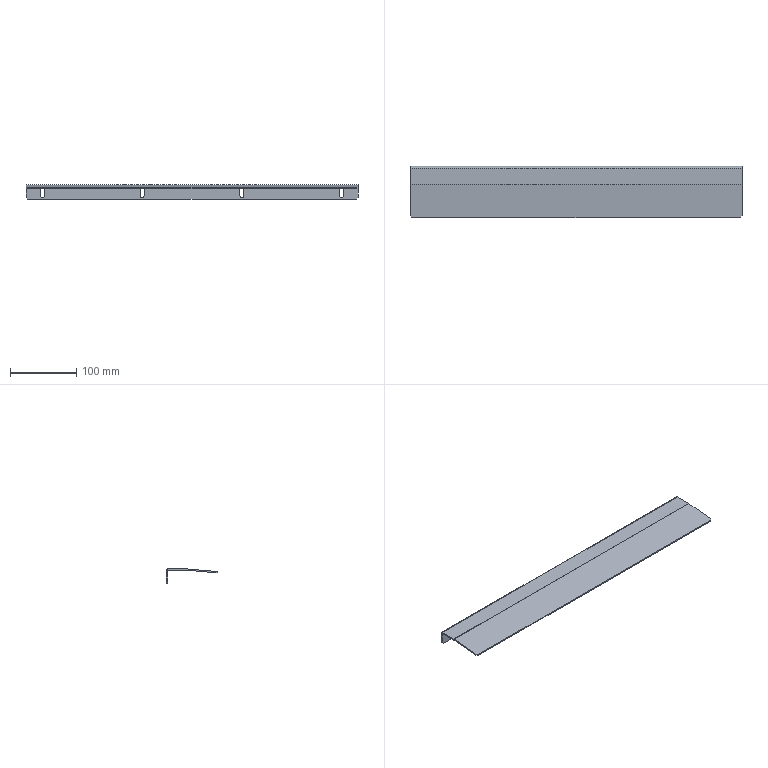Part | NX | 1 solid | 42 faces | box 500 x 76.984 x 22 mm | volume 95676 mm3 | plane 30 | cylinder 12 | commonest cylinder face diameters 5.5 x8 1.473 x2 5.473 x2
STEP:
#1=CARTESIAN_POINT('',(250.,-12.468,-2.));
#2=VERTEX_POINT('',#1);
#3=CARTESIAN_POINT('',(250.,11.763,-2.));
#4=VERTEX_POINT('',#3);
#5=CARTESIAN_POINT('',(250.,-12.5,-2.));
#6=DIRECTION('',(0.,1.,0.));
#7=VECTOR('',#6,1000.);
#8=LINE('',#5,#7);
#9=EDGE_CURVE('',#2,#4,#8,.T.);
#10=ORIENTED_EDGE('',*,*,#9,.F.);
#11=CARTESIAN_POINT('',(-250.,-12.468,-2.));
#12=VERTEX_POINT('',#11);
#13=CARTESIAN_POINT('',(-250.,-12.468,-2.));
#14=DIRECTION('',(-1.,0.,0.));
#15=VECTOR('',#14,1000.);
#16=LINE('',#13,#15);
#17=EDGE_CURVE('',#12,#2,#16,.F.);
#18=ORIENTED_EDGE('',*,*,#17,.F.);
#19=CARTESIAN_POINT('',(-250.,11.763,-2.));
#20=VERTEX_POINT('',#19);
#21=CARTESIAN_POINT('',(-250.,-12.5,-2.));
#22=DIRECTION('',(0.,-1.,0.));
#23=VECTOR('',#22,1000.);
#24=LINE('',#21,#23);
#25=EDGE_CURVE('',#20,#12,#24,.T.);
#26=ORIENTED_EDGE('',*,*,#25,.F.);
#27=CARTESIAN_POINT('',(250.,11.763,-2.));
#28=DIRECTION('',(1.,0.,0.));
#29=VECTOR('',#28,1000.);
#30=LINE('',#27,#29);
#31=EDGE_CURVE('',#4,#20,#30,.F.);
#32=ORIENTED_EDGE('',*,*,#31,.F.);
#33=EDGE_LOOP('',(#10,#18,#26,#32));
#34=FACE_BOUND('',#33,.T.);
#35=CARTESIAN_POINT('',(0.,0.,-2.));
#36=DIRECTION('',(0.,0.,-1.));
#37=DIRECTION('',(-1.,0.,0.));
#38=AXIS2_PLACEMENT_3D('',#35,#36,#37);
#39=PLANE('',#38);
#40=ADVANCED_FACE('',(#34),#39,.T.);
#41=CARTESIAN_POINT('',(-250.,-12.468,0.));
#42=VERTEX_POINT('',#41);
#43=CARTESIAN_POINT('',(250.,-12.468,0.));
#44=VERTEX_POINT('',#43);
#45=CARTESIAN_POINT('',(-250.,-12.468,0.));
#46=DIRECTION('',(-1.,0.,0.));
#47=VECTOR('',#46,1000.);
#48=LINE('',#45,#47);
#49=EDGE_CURVE('',#42,#44,#48,.F.);
#50=ORIENTED_EDGE('',*,*,#49,.T.);
#51=CARTESIAN_POINT('',(250.,11.763,0.));
#52=VERTEX_POINT('',#51);
#53=CARTESIAN_POINT('',(250.,-12.5,0.));
#54=DIRECTION('',(0.,1.,0.));
#55=VECTOR('',#54,1000.);
#56=LINE('',#53,#55);
#57=EDGE_CURVE('',#44,#52,#56,.T.);
#58=ORIENTED_EDGE('',*,*,#57,.T.);
#59=CARTESIAN_POINT('',(-250.,11.763,0.));
#60=VERTEX_POINT('',#59);
#61=CARTESIAN_POINT('',(250.,11.763,0.));
#62=DIRECTION('',(1.,0.,0.));
#63=VECTOR('',#62,1000.);
#64=LINE('',#61,#63);
#65=EDGE_CURVE('',#52,#60,#64,.F.);
#66=ORIENTED_EDGE('',*,*,#65,.T.);
#67=CARTESIAN_POINT('',(-250.,-12.5,0.));
#68=DIRECTION('',(0.,-1.,0.));
#69=VECTOR('',#68,1000.);
#70=LINE('',#67,#69);
#71=EDGE_CURVE('',#60,#42,#70,.T.);
#72=ORIENTED_EDGE('',*,*,#71,.T.);
#73=EDGE_LOOP('',(#50,#58,#66,#72));
#74=FACE_BOUND('',#73,.T.);
#75=CARTESIAN_POINT('',(0.,0.,0.));
#76=DIRECTION('',(0.,0.,-1.));
#77=DIRECTION('',(-1.,0.,0.));
#78=AXIS2_PLACEMENT_3D('',#75,#76,#77);
#79=PLANE('',#78);
#80=ADVANCED_FACE('',(#74),#79,.F.);
#81=ORIENTED_EDGE('',*,*,#25,.T.);
#82=CARTESIAN_POINT('',(-250.,-12.468,-2.));
#83=DIRECTION('',(0.,0.,1.));
#84=VECTOR('',#83,1000.);
#85=LINE('',#82,#84);
#86=EDGE_CURVE('',#12,#42,#85,.T.);
#87=ORIENTED_EDGE('',*,*,#86,.T.);
#88=ORIENTED_EDGE('',*,*,#71,.F.);
#89=CARTESIAN_POINT('',(-250.,11.763,-2.));
#90=DIRECTION('',(0.,0.,1.));
#91=VECTOR('',#90,1000.);
#92=LINE('',#89,#91);
#93=EDGE_CURVE('',#20,#60,#92,.T.);
#94=ORIENTED_EDGE('',*,*,#93,.F.);
#95=EDGE_LOOP('',(#81,#87,#88,#94));
#96=FACE_BOUND('',#95,.T.);
#97=CARTESIAN_POINT('',(-250.,-12.5,-2.));
#98=DIRECTION('',(-1.,0.,0.));
#99=DIRECTION('',(0.,0.,1.));
#100=AXIS2_PLACEMENT_3D('',#97,#98,#99);
#101=PLANE('',#100);
#102=ADVANCED_FACE('',(#96),#101,.T.);
#103=CARTESIAN_POINT('',(250.,-12.468,-2.));
#104=DIRECTION('',(0.,0.,1.));
#105=VECTOR('',#104,1000.);
#106=LINE('',#103,#105);
#107=EDGE_CURVE('',#2,#44,#106,.T.);
#108=ORIENTED_EDGE('',*,*,#107,.F.);
#109=ORIENTED_EDGE('',*,*,#9,.T.);
#110=CARTESIAN_POINT('',(250.,11.763,-2.));
#111=DIRECTION('',(0.,0.,1.));
#112=VECTOR('',#111,1000.);
#113=LINE('',#110,#112);
#114=EDGE_CURVE('',#4,#52,#113,.T.);
#115=ORIENTED_EDGE('',*,*,#114,.T.);
#116=ORIENTED_EDGE('',*,*,#57,.F.);
#117=EDGE_LOOP('',(#108,#109,#115,#116));
#118=FACE_BOUND('',#117,.T.);
#119=CARTESIAN_POINT('',(250.,-12.5,-2.));
#120=DIRECTION('',(1.,0.,0.));
#121=DIRECTION('',(0.,0.,-1.));
#122=AXIS2_PLACEMENT_3D('',#119,#120,#121);
#123=PLANE('',#122);
#124=ADVANCED_FACE('',(#118),#123,.T.);
#125=CARTESIAN_POINT('',(-250.,12.5,-2.737));
#126=VERTEX_POINT('',#125);
#127=CARTESIAN_POINT('',(-250.,14.5,-2.737));
#128=VERTEX_POINT('',#127);
#129=CARTESIAN_POINT('',(-250.,12.5,-2.737));
#130=DIRECTION('',(0.,1.,0.));
#131=VECTOR('',#130,1000.);
#132=LINE('',#129,#131);
#133=EDGE_CURVE('',#126,#128,#132,.T.);
#134=ORIENTED_EDGE('',*,*,#133,.F.);
#135=CARTESIAN_POINT('',(-250.,11.763,-2.737));
#136=DIRECTION('',(1.,0.,0.));
#137=DIRECTION('',(0.,0.,-1.));
#138=AXIS2_PLACEMENT_3D('',#135,#136,#137);
#139=CIRCLE('',#138,0.7366);
#140=EDGE_CURVE('',#20,#126,#139,.F.);
#141=ORIENTED_EDGE('',*,*,#140,.F.);
#142=ORIENTED_EDGE('',*,*,#93,.T.);
#143=CARTESIAN_POINT('',(-250.,11.763,-2.737));
#144=DIRECTION('',(1.,0.,0.));
#145=DIRECTION('',(0.,0.,-1.));
#146=AXIS2_PLACEMENT_3D('',#143,#144,#145);
#147=CIRCLE('',#146,2.737);
#148=EDGE_CURVE('',#60,#128,#147,.F.);
#149=ORIENTED_EDGE('',*,*,#148,.T.);
#150=EDGE_LOOP('',(#134,#141,#142,#149));
#151=FACE_BOUND('',#150,.T.);
#152=CARTESIAN_POINT('',(-250.,11.763,-2.737));
#153=DIRECTION('',(-1.,0.,0.));
#154=DIRECTION('',(0.,0.,1.));
#155=AXIS2_PLACEMENT_3D('',#152,#153,#154);
#156=PLANE('',#155);
#157=ADVANCED_FACE('',(#151),#156,.T.);
#158=CARTESIAN_POINT('',(250.,12.5,-2.737));
#159=VERTEX_POINT('',#158);
#160=CARTESIAN_POINT('',(250.,11.763,-2.737));
#161=DIRECTION('',(1.,0.,0.));
#162=DIRECTION('',(0.,0.,-1.));
#163=AXIS2_PLACEMENT_3D('',#160,#161,#162);
#164=CIRCLE('',#163,0.7366);
#165=EDGE_CURVE('',#159,#4,#164,.T.);
#166=ORIENTED_EDGE('',*,*,#165,.F.);
#167=CARTESIAN_POINT('',(250.,14.5,-2.737));
#168=VERTEX_POINT('',#167);
#169=CARTESIAN_POINT('',(250.,12.5,-2.737));
#170=DIRECTION('',(0.,1.,0.));
#171=VECTOR('',#170,1000.);
#172=LINE('',#169,#171);
#173=EDGE_CURVE('',#159,#168,#172,.T.);
#174=ORIENTED_EDGE('',*,*,#173,.T.);
#175=CARTESIAN_POINT('',(250.,11.763,-2.737));
#176=DIRECTION('',(1.,0.,0.));
#177=DIRECTION('',(0.,0.,-1.));
#178=AXIS2_PLACEMENT_3D('',#175,#176,#177);
#179=CIRCLE('',#178,2.737);
#180=EDGE_CURVE('',#168,#52,#179,.T.);
#181=ORIENTED_EDGE('',*,*,#180,.T.);
#182=ORIENTED_EDGE('',*,*,#114,.F.);
#183=EDGE_LOOP('',(#166,#174,#181,#182));
#184=FACE_BOUND('',#183,.T.);
#185=CARTESIAN_POINT('',(250.,11.763,-2.737));
#186=DIRECTION('',(-1.,0.,0.));
#187=DIRECTION('',(0.,0.,1.));
#188=AXIS2_PLACEMENT_3D('',#185,#186,#187);
#189=PLANE('',#188);
#190=ADVANCED_FACE('',(#184),#189,.F.);
#191=ORIENTED_EDGE('',*,*,#65,.F.);
#192=ORIENTED_EDGE('',*,*,#180,.F.);
#193=CARTESIAN_POINT('',(0.,14.5,-2.737));
#194=DIRECTION('',(1.,0.,0.));
#195=VECTOR('',#194,1000.);
#196=LINE('',#193,#195);
#197=EDGE_CURVE('',#128,#168,#196,.T.);
#198=ORIENTED_EDGE('',*,*,#197,.F.);
#199=ORIENTED_EDGE('',*,*,#148,.F.);
#200=EDGE_LOOP('',(#191,#192,#198,#199));
#201=FACE_BOUND('',#200,.T.);
#202=CARTESIAN_POINT('',(250.,11.763,-2.737));
#203=DIRECTION('',(1.,0.,0.));
#204=DIRECTION('',(0.,1.,0.));
#205=AXIS2_PLACEMENT_3D('',#202,#203,#204);
#206=CYLINDRICAL_SURFACE('',#205,2.737);
#207=ADVANCED_FACE('',(#201),#206,.T.);
#208=ORIENTED_EDGE('',*,*,#31,.T.);
#209=ORIENTED_EDGE('',*,*,#140,.T.);
#210=CARTESIAN_POINT('',(-250.,12.5,-2.737));
#211=DIRECTION('',(1.,0.,0.));
#212=VECTOR('',#211,1000.);
#213=LINE('',#210,#212);
#214=EDGE_CURVE('',#126,#159,#213,.T.);
#215=ORIENTED_EDGE('',*,*,#214,.T.);
#216=ORIENTED_EDGE('',*,*,#165,.T.);
#217=EDGE_LOOP('',(#208,#209,#215,#216));
#218=FACE_BOUND('',#217,.T.);
#219=CARTESIAN_POINT('',(250.,11.763,-2.737));
#220=DIRECTION('',(1.,0.,0.));
#221=DIRECTION('',(0.,1.,0.));
#222=AXIS2_PLACEMENT_3D('',#219,#220,#221);
#223=CYLINDRICAL_SURFACE('',#222,0.7366);
#224=ADVANCED_FACE('',(#218),#223,.F.);
#225=CARTESIAN_POINT('',(250.,12.5,-19.));
#226=VERTEX_POINT('',#225);
#227=CARTESIAN_POINT('',(250.,12.5,-2.));
#228=DIRECTION('',(0.,0.,1.));
#229=VECTOR('',#228,1000.);
#230=LINE('',#227,#229);
#231=EDGE_CURVE('',#226,#159,#230,.T.);
#232=ORIENTED_EDGE('',*,*,#231,.F.);
#233=CARTESIAN_POINT('',(250.,14.5,-19.));
#234=VERTEX_POINT('',#233);
#235=CARTESIAN_POINT('',(250.,14.5,-19.));
#236=DIRECTION('',(0.,1.,0.));
#237=VECTOR('',#236,1000.);
#238=LINE('',#235,#237);
#239=EDGE_CURVE('',#226,#234,#238,.T.);
#240=ORIENTED_EDGE('',*,*,#239,.T.);
#241=CARTESIAN_POINT('',(250.,14.5,-2.));
#242=DIRECTION('',(0.,0.,1.));
#243=VECTOR('',#242,1000.);
#244=LINE('',#241,#243);
#245=EDGE_CURVE('',#234,#168,#244,.T.);
#246=ORIENTED_EDGE('',*,*,#245,.T.);
#247=ORIENTED_EDGE('',*,*,#173,.F.);
#248=EDGE_LOOP('',(#232,#240,#246,#247));
#249=FACE_BOUND('',#248,.T.);
#250=CARTESIAN_POINT('',(250.,14.5,-2.));
#251=DIRECTION('',(1.,0.,0.));
#252=DIRECTION('',(0.,0.,-1.));
#253=AXIS2_PLACEMENT_3D('',#250,#251,#252);
#254=PLANE('',#253);
#255=ADVANCED_FACE('',(#249),#254,.T.);
#256=CARTESIAN_POINT('',(-250.,14.5,-19.));
#257=VERTEX_POINT('',#256);
#258=CARTESIAN_POINT('',(-250.,14.5,-22.));
#259=DIRECTION('',(0.,0.,-1.));
#260=VECTOR('',#259,1000.);
#261=LINE('',#258,#260);
#262=EDGE_CURVE('',#128,#257,#261,.T.);
#263=ORIENTED_EDGE('',*,*,#262,.T.);
#264=CARTESIAN_POINT('',(-250.,12.5,-19.));
#265=VERTEX_POINT('',#264);
#266=CARTESIAN_POINT('',(-250.,14.5,-19.));
#267=DIRECTION('',(0.,-1.,0.));
#268=VECTOR('',#267,1000.);
#269=LINE('',#266,#268);
#270=EDGE_CURVE('',#257,#265,#269,.T.);
#271=ORIENTED_EDGE('',*,*,#270,.T.);
#272=CARTESIAN_POINT('',(-250.,12.5,-22.));
#273=DIRECTION('',(0.,0.,-1.));
#274=VECTOR('',#273,1000.);
#275=LINE('',#272,#274);
#276=EDGE_CURVE('',#126,#265,#275,.T.);
#277=ORIENTED_EDGE('',*,*,#276,.F.);
#278=ORIENTED_EDGE('',*,*,#133,.T.);
#279=EDGE_LOOP('',(#263,#271,#277,#278));
#280=FACE_BOUND('',#279,.T.);
#281=CARTESIAN_POINT('',(-250.,14.5,-22.));
#282=DIRECTION('',(-1.,0.,0.));
#283=DIRECTION('',(0.,0.,1.));
#284=AXIS2_PLACEMENT_3D('',#281,#282,#283);
#285=PLANE('',#284);
#286=ADVANCED_FACE('',(#280),#285,.T.);
#287=CARTESIAN_POINT('',(227.75,14.5,-17.));
#288=VERTEX_POINT('',#287);
#289=CARTESIAN_POINT('',(222.25,14.5,-17.));
#290=VERTEX_POINT('',#289);
#291=CARTESIAN_POINT('',(225.,14.5,-17.));
#292=DIRECTION('',(0.,1.,0.));
#293=DIRECTION('',(0.,0.,1.));
#294=AXIS2_PLACEMENT_3D('',#291,#292,#293);
#295=CIRCLE('',#294,2.75);
#296=EDGE_CURVE('',#288,#290,#295,.T.);
#297=ORIENTED_EDGE('',*,*,#296,.F.);
#298=CARTESIAN_POINT('',(227.75,14.5,-7.));
#299=VERTEX_POINT('',#298);
#300=CARTESIAN_POINT('',(227.75,14.5,-17.));
#301=DIRECTION('',(0.,0.,-1.));
#302=VECTOR('',#301,1000.);
#303=LINE('',#300,#302);
#304=EDGE_CURVE('',#299,#288,#303,.T.);
#305=ORIENTED_EDGE('',*,*,#304,.F.);
#306=CARTESIAN_POINT('',(222.25,14.5,-7.));
#307=VERTEX_POINT('',#306);
#308=CARTESIAN_POINT('',(225.,14.5,-7.));
#309=DIRECTION('',(0.,1.,0.));
#310=DIRECTION('',(0.,0.,1.));
#311=AXIS2_PLACEMENT_3D('',#308,#309,#310);
#312=CIRCLE('',#311,2.75);
#313=EDGE_CURVE('',#307,#299,#312,.T.);
#314=ORIENTED_EDGE('',*,*,#313,.F.);
#315=CARTESIAN_POINT('',(222.25,14.5,-17.));
#316=DIRECTION('',(0.,0.,1.));
#317=VECTOR('',#316,1000.);
#318=LINE('',#315,#317);
#319=EDGE_CURVE('',#290,#307,#318,.T.);
#320=ORIENTED_EDGE('',*,*,#319,.F.);
#321=EDGE_LOOP('',(#297,#305,#314,#320));
#322=FACE_BOUND('',#321,.T.);
#323=CARTESIAN_POINT('',(77.75,14.5,-17.));
#324=VERTEX_POINT('',#323);
#325=CARTESIAN_POINT('',(72.25,14.5,-17.));
#326=VERTEX_POINT('',#325);
#327=CARTESIAN_POINT('',(75.,14.5,-17.));
#328=DIRECTION('',(0.,1.,0.));
#329=DIRECTION('',(0.,0.,1.));
#330=AXIS2_PLACEMENT_3D('',#327,#328,#329);
#331=CIRCLE('',#330,2.75);
#332=EDGE_CURVE('',#324,#326,#331,.T.);
#333=ORIENTED_EDGE('',*,*,#332,.F.);
#334=CARTESIAN_POINT('',(77.75,14.5,-7.));
#335=VERTEX_POINT('',#334);
#336=CARTESIAN_POINT('',(77.75,14.5,-17.));
#337=DIRECTION('',(0.,0.,-1.));
#338=VECTOR('',#337,1000.);
#339=LINE('',#336,#338);
#340=EDGE_CURVE('',#335,#324,#339,.T.);
#341=ORIENTED_EDGE('',*,*,#340,.F.);
#342=CARTESIAN_POINT('',(72.25,14.5,-7.));
#343=VERTEX_POINT('',#342);
#344=CARTESIAN_POINT('',(75.,14.5,-7.));
#345=DIRECTION('',(0.,1.,0.));
#346=DIRECTION('',(0.,0.,1.));
#347=AXIS2_PLACEMENT_3D('',#344,#345,#346);
#348=CIRCLE('',#347,2.75);
#349=EDGE_CURVE('',#343,#335,#348,.T.);
#350=ORIENTED_EDGE('',*,*,#349,.F.);
#351=CARTESIAN_POINT('',(72.25,14.5,-17.));
#352=DIRECTION('',(0.,0.,1.));
#353=VECTOR('',#352,1000.);
#354=LINE('',#351,#353);
#355=EDGE_CURVE('',#326,#343,#354,.T.);
#356=ORIENTED_EDGE('',*,*,#355,.F.);
#357=EDGE_LOOP('',(#333,#341,#350,#356));
#358=FACE_BOUND('',#357,.T.);
#359=CARTESIAN_POINT('',(-72.25,14.5,-17.));
#360=VERTEX_POINT('',#359);
#361=CARTESIAN_POINT('',(-77.75,14.5,-17.));
#362=VERTEX_POINT('',#361);
#363=CARTESIAN_POINT('',(-75.,14.5,-17.));
#364=DIRECTION('',(0.,1.,0.));
#365=DIRECTION('',(0.,0.,1.));
#366=AXIS2_PLACEMENT_3D('',#363,#364,#365);
#367=CIRCLE('',#366,2.75);
#368=EDGE_CURVE('',#360,#362,#367,.T.);
#369=ORIENTED_EDGE('',*,*,#368,.F.);
#370=CARTESIAN_POINT('',(-72.25,14.5,-7.));
#371=VERTEX_POINT('',#370);
#372=CARTESIAN_POINT('',(-72.25,14.5,-17.));
#373=DIRECTION('',(0.,0.,-1.));
#374=VECTOR('',#373,1000.);
#375=LINE('',#372,#374);
#376=EDGE_CURVE('',#371,#360,#375,.T.);
#377=ORIENTED_EDGE('',*,*,#376,.F.);
#378=CARTESIAN_POINT('',(-77.75,14.5,-7.));
#379=VERTEX_POINT('',#378);
#380=CARTESIAN_POINT('',(-75.,14.5,-7.));
#381=DIRECTION('',(0.,1.,0.));
#382=DIRECTION('',(0.,0.,1.));
#383=AXIS2_PLACEMENT_3D('',#380,#381,#382);
#384=CIRCLE('',#383,2.75);
#385=EDGE_CURVE('',#379,#371,#384,.T.);
#386=ORIENTED_EDGE('',*,*,#385,.F.);
#387=CARTESIAN_POINT('',(-77.75,14.5,-17.));
#388=DIRECTION('',(0.,0.,1.));
#389=VECTOR('',#388,1000.);
#390=LINE('',#387,#389);
#391=EDGE_CURVE('',#362,#379,#390,.T.);
#392=ORIENTED_EDGE('',*,*,#391,.F.);
#393=EDGE_LOOP('',(#369,#377,#386,#392));
#394=FACE_BOUND('',#393,.T.);
#395=CARTESIAN_POINT('',(-222.25,14.5,-17.));
#396=VERTEX_POINT('',#395);
#397=CARTESIAN_POINT('',(-227.75,14.5,-17.));
#398=VERTEX_POINT('',#397);
#399=CARTESIAN_POINT('',(-225.,14.5,-17.));
#400=DIRECTION('',(0.,1.,0.));
#401=DIRECTION('',(0.,0.,1.));
#402=AXIS2_PLACEMENT_3D('',#399,#400,#401);
#403=CIRCLE('',#402,2.75);
#404=EDGE_CURVE('',#396,#398,#403,.T.);
#405=ORIENTED_EDGE('',*,*,#404,.F.);
#406=CARTESIAN_POINT('',(-222.25,14.5,-7.));
#407=VERTEX_POINT('',#406);
#408=CARTESIAN_POINT('',(-222.25,14.5,-17.));
#409=DIRECTION('',(0.,0.,-1.));
#410=VECTOR('',#409,1000.);
#411=LINE('',#408,#410);
#412=EDGE_CURVE('',#407,#396,#411,.T.);
#413=ORIENTED_EDGE('',*,*,#412,.F.);
#414=CARTESIAN_POINT('',(-227.75,14.5,-7.));
#415=VERTEX_POINT('',#414);
#416=CARTESIAN_POINT('',(-225.,14.5,-7.));
#417=DIRECTION('',(0.,1.,0.));
#418=DIRECTION('',(0.,0.,1.));
#419=AXIS2_PLACEMENT_3D('',#416,#417,#418);
#420=CIRCLE('',#419,2.75);
#421=EDGE_CURVE('',#415,#407,#420,.T.);
#422=ORIENTED_EDGE('',*,*,#421,.F.);
#423=CARTESIAN_POINT('',(-227.75,14.5,-17.));
#424=DIRECTION('',(0.,0.,1.));
#425=VECTOR('',#424,1000.);
#426=LINE('',#423,#425);
#427=EDGE_CURVE('',#398,#415,#426,.T.);
#428=ORIENTED_EDGE('',*,*,#427,.F.);
#429=EDGE_LOOP('',(#405,#413,#422,#428));
#430=FACE_BOUND('',#429,.T.);
#431=CARTESIAN_POINT('',(-247.,14.5,-22.));
#432=VERTEX_POINT('',#431);
#433=CARTESIAN_POINT('',(247.,14.5,-22.));
#434=VERTEX_POINT('',#433);
#435=CARTESIAN_POINT('',(250.,14.5,-22.));
#436=DIRECTION('',(1.,0.,0.));
#437=VECTOR('',#436,1000.);
#438=LINE('',#435,#437);
#439=EDGE_CURVE('',#432,#434,#438,.T.);
#440=ORIENTED_EDGE('',*,*,#439,.F.);
#441=CARTESIAN_POINT('',(-134.5,14.5,-134.5));
#442=DIRECTION('',(0.7071,0.,-0.7071));
#443=VECTOR('',#442,1000.);
#444=LINE('',#441,#443);
#445=EDGE_CURVE('',#432,#257,#444,.F.);
#446=ORIENTED_EDGE('',*,*,#445,.T.);
#447=ORIENTED_EDGE('',*,*,#262,.F.);
#448=ORIENTED_EDGE('',*,*,#197,.T.);
#449=ORIENTED_EDGE('',*,*,#245,.F.);
#450=CARTESIAN_POINT('',(134.5,14.5,-134.5));
#451=DIRECTION('',(0.7071,0.,0.7071));
#452=VECTOR('',#451,1000.);
#453=LINE('',#450,#452);
#454=EDGE_CURVE('',#234,#434,#453,.F.);
#455=ORIENTED_EDGE('',*,*,#454,.T.);
#456=EDGE_LOOP('',(#440,#446,#447,#448,#449,#455));
#457=FACE_BOUND('',#456,.T.);
#458=CARTESIAN_POINT('',(0.,14.5,0.));
#459=DIRECTION('',(0.,1.,0.));
#460=DIRECTION('',(0.,0.,1.));
#461=AXIS2_PLACEMENT_3D('',#458,#459,#460);
#462=PLANE('',#461);
#463=ADVANCED_FACE('',(#322,#358,#394,#430,#457),#462,.T.);
#464=CARTESIAN_POINT('',(227.75,12.5,-17.));
#465=VERTEX_POINT('',#464);
#466=CARTESIAN_POINT('',(227.75,12.5,-7.));
#467=VERTEX_POINT('',#466);
#468=CARTESIAN_POINT('',(227.75,12.5,-17.));
#469=DIRECTION('',(0.,0.,1.));
#470=VECTOR('',#469,1000.);
#471=LINE('',#468,#470);
#472=EDGE_CURVE('',#465,#467,#471,.T.);
#473=ORIENTED_EDGE('',*,*,#472,.F.);
#474=CARTESIAN_POINT('',(222.25,12.5,-17.));
#475=VERTEX_POINT('',#474);
#476=CARTESIAN_POINT('',(225.,12.5,-17.));
#477=DIRECTION('',(0.,1.,0.));
#478=DIRECTION('',(0.,0.,1.));
#479=AXIS2_PLACEMENT_3D('',#476,#477,#478);
#480=CIRCLE('',#479,2.75);
#481=EDGE_CURVE('',#475,#465,#480,.F.);
#482=ORIENTED_EDGE('',*,*,#481,.F.);
#483=CARTESIAN_POINT('',(222.25,12.5,-7.));
#484=VERTEX_POINT('',#483);
#485=CARTESIAN_POINT('',(222.25,12.5,-17.));
#486=DIRECTION('',(0.,0.,-1.));
#487=VECTOR('',#486,1000.);
#488=LINE('',#485,#487);
#489=EDGE_CURVE('',#484,#475,#488,.T.);
#490=ORIENTED_EDGE('',*,*,#489,.F.);
#491=CARTESIAN_POINT('',(225.,12.5,-7.));
#492=DIRECTION('',(0.,1.,0.));
#493=DIRECTION('',(0.,0.,1.));
#494=AXIS2_PLACEMENT_3D('',#491,#492,#493);
#495=CIRCLE('',#494,2.75);
#496=EDGE_CURVE('',#467,#484,#495,.F.);
#497=ORIENTED_EDGE('',*,*,#496,.F.);
#498=EDGE_LOOP('',(#473,#482,#490,#497));
#499=FACE_BOUND('',#498,.T.);
#500=CARTESIAN_POINT('',(77.75,12.5,-17.));
#501=VERTEX_POINT('',#500);
#502=CARTESIAN_POINT('',(77.75,12.5,-7.));
#503=VERTEX_POINT('',#502);
#504=CARTESIAN_POINT('',(77.75,12.5,-17.));
#505=DIRECTION('',(0.,0.,1.));
#506=VECTOR('',#505,1000.);
#507=LINE('',#504,#506);
#508=EDGE_CURVE('',#501,#503,#507,.T.);
#509=ORIENTED_EDGE('',*,*,#508,.F.);
#510=CARTESIAN_POINT('',(72.25,12.5,-17.));
#511=VERTEX_POINT('',#510);
#512=CARTESIAN_POINT('',(75.,12.5,-17.));
#513=DIRECTION('',(0.,1.,0.));
#514=DIRECTION('',(0.,0.,1.));
#515=AXIS2_PLACEMENT_3D('',#512,#513,#514);
#516=CIRCLE('',#515,2.75);
#517=EDGE_CURVE('',#511,#501,#516,.F.);
#518=ORIENTED_EDGE('',*,*,#517,.F.);
#519=CARTESIAN_POINT('',(72.25,12.5,-7.));
#520=VERTEX_POINT('',#519);
#521=CARTESIAN_POINT('',(72.25,12.5,-17.));
#522=DIRECTION('',(0.,0.,-1.));
#523=VECTOR('',#522,1000.);
#524=LINE('',#521,#523);
#525=EDGE_CURVE('',#520,#511,#524,.T.);
#526=ORIENTED_EDGE('',*,*,#525,.F.);
#527=CARTESIAN_POINT('',(75.,12.5,-7.));
#528=DIRECTION('',(0.,1.,0.));
#529=DIRECTION('',(0.,0.,1.));
#530=AXIS2_PLACEMENT_3D('',#527,#528,#529);
#531=CIRCLE('',#530,2.75);
#532=EDGE_CURVE('',#503,#520,#531,.F.);
#533=ORIENTED_EDGE('',*,*,#532,.F.);
#534=EDGE_LOOP('',(#509,#518,#526,#533));
#535=FACE_BOUND('',#534,.T.);
#536=CARTESIAN_POINT('',(-72.25,12.5,-17.));
#537=VERTEX_POINT('',#536);
#538=CARTESIAN_POINT('',(-72.25,12.5,-7.));
#539=VERTEX_POINT('',#538);
#540=CARTESIAN_POINT('',(-72.25,12.5,-17.));
#541=DIRECTION('',(0.,0.,1.));
#542=VECTOR('',#541,1000.);
#543=LINE('',#540,#542);
#544=EDGE_CURVE('',#537,#539,#543,.T.);
#545=ORIENTED_EDGE('',*,*,#544,.F.);
#546=CARTESIAN_POINT('',(-77.75,12.5,-17.));
#547=VERTEX_POINT('',#546);
#548=CARTESIAN_POINT('',(-75.,12.5,-17.));
#549=DIRECTION('',(0.,1.,0.));
#550=DIRECTION('',(0.,0.,1.));
#551=AXIS2_PLACEMENT_3D('',#548,#549,#550);
#552=CIRCLE('',#551,2.75);
#553=EDGE_CURVE('',#547,#537,#552,.F.);
#554=ORIENTED_EDGE('',*,*,#553,.F.);
#555=CARTESIAN_POINT('',(-77.75,12.5,-7.));
#556=VERTEX_POINT('',#555);
#557=CARTESIAN_POINT('',(-77.75,12.5,-17.));
#558=DIRECTION('',(0.,0.,-1.));
#559=VECTOR('',#558,1000.);
#560=LINE('',#557,#559);
#561=EDGE_CURVE('',#556,#547,#560,.T.);
#562=ORIENTED_EDGE('',*,*,#561,.F.);
#563=CARTESIAN_POINT('',(-75.,12.5,-7.));
#564=DIRECTION('',(0.,1.,0.));
#565=DIRECTION('',(0.,0.,1.));
#566=AXIS2_PLACEMENT_3D('',#563,#564,#565);
#567=CIRCLE('',#566,2.75);
#568=EDGE_CURVE('',#539,#556,#567,.F.);
#569=ORIENTED_EDGE('',*,*,#568,.F.);
#570=EDGE_LOOP('',(#545,#554,#562,#569));
#571=FACE_BOUND('',#570,.T.);
#572=CARTESIAN_POINT('',(-222.25,12.5,-17.));
#573=VERTEX_POINT('',#572);
#574=CARTESIAN_POINT('',(-222.25,12.5,-7.));
#575=VERTEX_POINT('',#574);
#576=CARTESIAN_POINT('',(-222.25,12.5,-17.));
#577=DIRECTION('',(0.,0.,1.));
#578=VECTOR('',#577,1000.);
#579=LINE('',#576,#578);
#580=EDGE_CURVE('',#573,#575,#579,.T.);
#581=ORIENTED_EDGE('',*,*,#580,.F.);
#582=CARTESIAN_POINT('',(-227.75,12.5,-17.));
#583=VERTEX_POINT('',#582);
#584=CARTESIAN_POINT('',(-225.,12.5,-17.));
#585=DIRECTION('',(0.,1.,0.));
#586=DIRECTION('',(0.,0.,1.));
#587=AXIS2_PLACEMENT_3D('',#584,#585,#586);
#588=CIRCLE('',#587,2.75);
#589=EDGE_CURVE('',#583,#573,#588,.F.);
#590=ORIENTED_EDGE('',*,*,#589,.F.);
#591=CARTESIAN_POINT('',(-227.75,12.5,-7.));
#592=VERTEX_POINT('',#591);
#593=CARTESIAN_POINT('',(-227.75,12.5,-17.));
#594=DIRECTION('',(0.,0.,-1.));
#595=VECTOR('',#594,1000.);
#596=LINE('',#593,#595);
#597=EDGE_CURVE('',#592,#583,#596,.T.);
#598=ORIENTED_EDGE('',*,*,#597,.F.);
#599=CARTESIAN_POINT('',(-225.,12.5,-7.));
#600=DIRECTION('',(0.,1.,0.));
#601=DIRECTION('',(0.,0.,1.));
#602=AXIS2_PLACEMENT_3D('',#599,#600,#601);
#603=CIRCLE('',#602,2.75);
#604=EDGE_CURVE('',#575,#592,#603,.F.);
#605=ORIENTED_EDGE('',*,*,#604,.F.);
#606=EDGE_LOOP('',(#581,#590,#598,#605));
#607=FACE_BOUND('',#606,.T.);
#608=ORIENTED_EDGE('',*,*,#276,.T.);
#609=CARTESIAN_POINT('',(-247.,12.5,-22.));
#610=VERTEX_POINT('',#609);
#611=CARTESIAN_POINT('',(-250.,12.5,-19.));
#612=DIRECTION('',(-0.7071,0.,0.7071));
#613=VECTOR('',#612,1000.);
#614=LINE('',#611,#613);
#615=EDGE_CURVE('',#265,#610,#614,.F.);
#616=ORIENTED_EDGE('',*,*,#615,.T.);
#617=CARTESIAN_POINT('',(247.,12.5,-22.));
#618=VERTEX_POINT('',#617);
#619=CARTESIAN_POINT('',(250.,12.5,-22.));
#620=DIRECTION('',(1.,0.,0.));
#621=VECTOR('',#620,1000.);
#622=LINE('',#619,#621);
#623=EDGE_CURVE('',#610,#618,#622,.T.);
#624=ORIENTED_EDGE('',*,*,#623,.T.);
#625=CARTESIAN_POINT('',(247.,12.5,-22.));
#626=DIRECTION('',(-0.7071,0.,-0.7071));
#627=VECTOR('',#626,1000.);
#628=LINE('',#625,#627);
#629=EDGE_CURVE('',#618,#226,#628,.F.);
#630=ORIENTED_EDGE('',*,*,#629,.T.);
#631=ORIENTED_EDGE('',*,*,#231,.T.);
#632=ORIENTED_EDGE('',*,*,#214,.F.);
#633=EDGE_LOOP('',(#608,#616,#624,#630,#631,#632));
#634=FACE_BOUND('',#633,.T.);
#635=CARTESIAN_POINT('',(0.,12.5,0.));
#636=DIRECTION('',(0.,1.,0.));
#637=DIRECTION('',(0.,0.,1.));
#638=AXIS2_PLACEMENT_3D('',#635,#636,#637);
#639=PLANE('',#638);
#640=ADVANCED_FACE('',(#499,#535,#571,#607,#634),#639,.F.);
#641=ORIENTED_EDGE('',*,*,#623,.F.);
#642=CARTESIAN_POINT('',(-247.,14.5,-22.));
#643=DIRECTION('',(0.,1.,0.));
#644=VECTOR('',#643,1000.);
#645=LINE('',#642,#644);
#646=EDGE_CURVE('',#610,#432,#645,.T.);
#647=ORIENTED_EDGE('',*,*,#646,.T.);
#648=ORIENTED_EDGE('',*,*,#439,.T.);
#649=CARTESIAN_POINT('',(247.,14.5,-22.));
#650=DIRECTION('',(0.,-1.,0.));
#651=VECTOR('',#650,1000.);
#652=LINE('',#649,#651);
#653=EDGE_CURVE('',#434,#618,#652,.T.);
#654=ORIENTED_EDGE('',*,*,#653,.T.);
#655=EDGE_LOOP('',(#641,#647,#648,#654));
#656=FACE_BOUND('',#655,.T.);
#657=CARTESIAN_POINT('',(250.,14.5,-22.));
#658=DIRECTION('',(0.,0.,-1.));
#659=DIRECTION('',(0.,1.,0.));
#660=AXIS2_PLACEMENT_3D('',#657,#658,#659);
#661=PLANE('',#660);
#662=ADVANCED_FACE('',(#656),#661,.T.);
#663=CARTESIAN_POINT('',(250.,-12.532,-2.003));
#664=VERTEX_POINT('',#663);
#665=CARTESIAN_POINT('',(250.,-12.706,-0.01041));
#666=VERTEX_POINT('',#665);
#667=CARTESIAN_POINT('',(250.,-12.532,-2.003));
#668=DIRECTION('',(0.,-0.08716,0.9962));
#669=VECTOR('',#668,1000.);
#670=LINE('',#667,#669);
#671=EDGE_CURVE('',#664,#666,#670,.T.);
#672=ORIENTED_EDGE('',*,*,#671,.F.);
#673=CARTESIAN_POINT('',(250.,-12.468,-2.737));
#674=DIRECTION('',(-1.,0.,0.));
#675=DIRECTION('',(0.,0.,1.));
#676=AXIS2_PLACEMENT_3D('',#673,#674,#675);
#677=CIRCLE('',#676,0.7366);
#678=EDGE_CURVE('',#2,#664,#677,.F.);
#679=ORIENTED_EDGE('',*,*,#678,.F.);
#680=ORIENTED_EDGE('',*,*,#107,.T.);
#681=CARTESIAN_POINT('',(250.,-12.468,-2.737));
#682=DIRECTION('',(-1.,0.,0.));
#683=DIRECTION('',(0.,0.,1.));
#684=AXIS2_PLACEMENT_3D('',#681,#682,#683);
#685=CIRCLE('',#684,2.737);
#686=EDGE_CURVE('',#44,#666,#685,.F.);
#687=ORIENTED_EDGE('',*,*,#686,.T.);
#688=EDGE_LOOP('',(#672,#679,#680,#687));
#689=FACE_BOUND('',#688,.T.);
#690=CARTESIAN_POINT('',(250.,-12.468,-2.737));
#691=DIRECTION('',(1.,0.,0.));
#692=DIRECTION('',(0.,0.,-1.));
#693=AXIS2_PLACEMENT_3D('',#690,#691,#692);
#694=PLANE('',#693);
#695=ADVANCED_FACE('',(#689),#694,.T.);
#696=CARTESIAN_POINT('',(-250.,-12.532,-2.003));
#697=VERTEX_POINT('',#696);
#698=CARTESIAN_POINT('',(-250.,-12.468,-2.737));
#699=DIRECTION('',(-1.,0.,0.));
#700=DIRECTION('',(0.,0.,1.));
#701=AXIS2_PLACEMENT_3D('',#698,#699,#700);
#702=CIRCLE('',#701,0.7366);
#703=EDGE_CURVE('',#697,#12,#702,.T.);
#704=ORIENTED_EDGE('',*,*,#703,.F.);
#705=CARTESIAN_POINT('',(-250.,-12.706,-0.01041));
#706=VERTEX_POINT('',#705);
#707=CARTESIAN_POINT('',(-250.,-12.532,-2.003));
#708=DIRECTION('',(0.,-0.08716,0.9962));
#709=VECTOR('',#708,1000.);
#710=LINE('',#707,#709);
#711=EDGE_CURVE('',#697,#706,#710,.T.);
#712=ORIENTED_EDGE('',*,*,#711,.T.);
#713=CARTESIAN_POINT('',(-250.,-12.468,-2.737));
#714=DIRECTION('',(-1.,0.,0.));
#715=DIRECTION('',(0.,0.,1.));
#716=AXIS2_PLACEMENT_3D('',#713,#714,#715);
#717=CIRCLE('',#716,2.737);
#718=EDGE_CURVE('',#706,#42,#717,.T.);
#719=ORIENTED_EDGE('',*,*,#718,.T.);
#720=ORIENTED_EDGE('',*,*,#86,.F.);
#721=EDGE_LOOP('',(#704,#712,#719,#720));
#722=FACE_BOUND('',#721,.T.);
#723=CARTESIAN_POINT('',(-250.,-12.468,-2.737));
#724=DIRECTION('',(1.,0.,0.));
#725=DIRECTION('',(0.,0.,-1.));
#726=AXIS2_PLACEMENT_3D('',#723,#724,#725);
#727=PLANE('',#726);
#728=ADVANCED_FACE('',(#722),#727,.F.);
#729=ORIENTED_EDGE('',*,*,#49,.F.);
#730=ORIENTED_EDGE('',*,*,#718,.F.);
#731=CARTESIAN_POINT('',(0.,-12.706,-0.01041));
#732=DIRECTION('',(-1.,0.,0.));
#733=VECTOR('',#732,1000.);
#734=LINE('',#731,#733);
#735=EDGE_CURVE('',#666,#706,#734,.T.);
#736=ORIENTED_EDGE('',*,*,#735,.F.);
#737=ORIENTED_EDGE('',*,*,#686,.F.);
#738=EDGE_LOOP('',(#729,#730,#736,#737));
#739=FACE_BOUND('',#738,.T.);
#740=CARTESIAN_POINT('',(-250.,-12.468,-2.737));
#741=DIRECTION('',(-1.,0.,0.));
#742=DIRECTION('',(0.,-0.08716,0.9962));
#743=AXIS2_PLACEMENT_3D('',#740,#741,#742);
#744=CYLINDRICAL_SURFACE('',#743,2.737);
#745=ADVANCED_FACE('',(#739),#744,.T.);
#746=ORIENTED_EDGE('',*,*,#17,.T.);
#747=ORIENTED_EDGE('',*,*,#678,.T.);
#748=CARTESIAN_POINT('',(250.,-12.532,-2.003));
#749=DIRECTION('',(-1.,0.,0.));
#750=VECTOR('',#749,1000.);
#751=LINE('',#748,#750);
#752=EDGE_CURVE('',#664,#697,#751,.T.);
#753=ORIENTED_EDGE('',*,*,#752,.T.);
#754=ORIENTED_EDGE('',*,*,#703,.T.);
#755=EDGE_LOOP('',(#746,#747,#753,#754));
#756=FACE_BOUND('',#755,.T.);
#757=CARTESIAN_POINT('',(-250.,-12.468,-2.737));
#758=DIRECTION('',(-1.,0.,0.));
#759=DIRECTION('',(0.,-0.08716,0.9962));
#760=AXIS2_PLACEMENT_3D('',#757,#758,#759);
#761=CYLINDRICAL_SURFACE('',#760,0.7366);
#762=ADVANCED_FACE('',(#756),#761,.F.);
#763=CARTESIAN_POINT('',(-250.,-59.321,-6.096));
#764=VERTEX_POINT('',#763);
#765=CARTESIAN_POINT('',(-250.,-12.5,-2.));
#766=DIRECTION('',(0.,0.9962,0.08716));
#767=VECTOR('',#766,1000.);
#768=LINE('',#765,#767);
#769=EDGE_CURVE('',#764,#697,#768,.T.);
#770=ORIENTED_EDGE('',*,*,#769,.F.);
#771=CARTESIAN_POINT('',(-250.,-59.495,-4.104));
#772=VERTEX_POINT('',#771);
#773=CARTESIAN_POINT('',(-250.,-59.495,-4.104));
#774=DIRECTION('',(0.,-0.08716,0.9962));
#775=VECTOR('',#774,1000.);
#776=LINE('',#773,#775);
#777=EDGE_CURVE('',#764,#772,#776,.T.);
#778=ORIENTED_EDGE('',*,*,#777,.T.);
#779=CARTESIAN_POINT('',(-250.,-12.674,-0.007611));
#780=DIRECTION('',(0.,0.9962,0.08716));
#781=VECTOR('',#780,1000.);
#782=LINE('',#779,#781);
#783=EDGE_CURVE('',#772,#706,#782,.T.);
#784=ORIENTED_EDGE('',*,*,#783,.T.);
#785=ORIENTED_EDGE('',*,*,#711,.F.);
#786=EDGE_LOOP('',(#770,#778,#784,#785));
#787=FACE_BOUND('',#786,.T.);
#788=CARTESIAN_POINT('',(-250.,-12.674,-0.007611));
#789=DIRECTION('',(-1.,0.,0.));
#790=DIRECTION('',(0.,0.,1.));
#791=AXIS2_PLACEMENT_3D('',#788,#789,#790);
#792=PLANE('',#791);
#793=ADVANCED_FACE('',(#787),#792,.T.);
#794=CARTESIAN_POINT('',(250.,-59.495,-4.104));
#795=VERTEX_POINT('',#794);
#796=CARTESIAN_POINT('',(250.,-62.484,-4.365));
#797=DIRECTION('',(0.,-0.9962,-0.08716));
#798=VECTOR('',#797,1000.);
#799=LINE('',#796,#798);
#800=EDGE_CURVE('',#666,#795,#799,.T.);
#801=ORIENTED_EDGE('',*,*,#800,.T.);
#802=CARTESIAN_POINT('',(250.,-59.321,-6.096));
#803=VERTEX_POINT('',#802);
#804=CARTESIAN_POINT('',(250.,-59.495,-4.104));
#805=DIRECTION('',(0.,0.08716,-0.9962));
#806=VECTOR('',#805,1000.);
#807=LINE('',#804,#806);
#808=EDGE_CURVE('',#795,#803,#807,.T.);
#809=ORIENTED_EDGE('',*,*,#808,.T.);
#810=CARTESIAN_POINT('',(250.,-62.31,-6.358));
#811=DIRECTION('',(0.,-0.9962,-0.08716));
#812=VECTOR('',#811,1000.);
#813=LINE('',#810,#812);
#814=EDGE_CURVE('',#664,#803,#813,.T.);
#815=ORIENTED_EDGE('',*,*,#814,.F.);
#816=ORIENTED_EDGE('',*,*,#671,.T.);
#817=EDGE_LOOP('',(#801,#809,#815,#816));
#818=FACE_BOUND('',#817,.T.);
#819=CARTESIAN_POINT('',(250.,-62.484,-4.365));
#820=DIRECTION('',(1.,0.,0.));
#821=DIRECTION('',(0.,0.,-1.));
#822=AXIS2_PLACEMENT_3D('',#819,#820,#821);
#823=PLANE('',#822);
#824=ADVANCED_FACE('',(#818),#823,.T.);
#825=CARTESIAN_POINT('',(247.,-62.484,-4.365));
#826=VERTEX_POINT('',#825);
#827=CARTESIAN_POINT('',(-247.,-62.484,-4.365));
#828=VERTEX_POINT('',#827);
#829=CARTESIAN_POINT('',(-250.,-62.484,-4.365));
#830=DIRECTION('',(-1.,0.,0.));
#831=VECTOR('',#830,1000.);
#832=LINE('',#829,#831);
#833=EDGE_CURVE('',#826,#828,#832,.T.);
#834=ORIENTED_EDGE('',*,*,#833,.F.);
#835=CARTESIAN_POINT('',(154.813,-154.32,-12.4));
#836=DIRECTION('',(-0.7071,-0.7044,-0.06163));
#837=VECTOR('',#836,1000.);
#838=LINE('',#835,#837);
#839=EDGE_CURVE('',#826,#795,#838,.F.);
#840=ORIENTED_EDGE('',*,*,#839,.T.);
#841=ORIENTED_EDGE('',*,*,#800,.F.);
#842=ORIENTED_EDGE('',*,*,#735,.T.);
#843=ORIENTED_EDGE('',*,*,#783,.F.);
#844=CARTESIAN_POINT('',(-154.813,-154.32,-12.4));
#845=DIRECTION('',(-0.7071,0.7044,0.06163));
#846=VECTOR('',#845,1000.);
#847=LINE('',#844,#846);
#848=EDGE_CURVE('',#772,#828,#847,.F.);
#849=ORIENTED_EDGE('',*,*,#848,.T.);
#850=EDGE_LOOP('',(#834,#840,#841,#842,#843,#849));
#851=FACE_BOUND('',#850,.T.);
#852=CARTESIAN_POINT('',(0.,-0.09561,1.093));
#853=DIRECTION('',(0.,-0.08716,0.9962));
#854=DIRECTION('',(0.,-0.9962,-0.08716));
#855=AXIS2_PLACEMENT_3D('',#852,#853,#854);
#856=PLANE('',#855);
#857=ADVANCED_FACE('',(#851),#856,.T.);
#858=ORIENTED_EDGE('',*,*,#814,.T.);
#859=CARTESIAN_POINT('',(247.,-62.31,-6.358));
#860=VERTEX_POINT('',#859);
#861=CARTESIAN_POINT('',(250.,-59.321,-6.096));
#862=DIRECTION('',(0.7071,0.7044,0.06163));
#863=VECTOR('',#862,1000.);
#864=LINE('',#861,#863);
#865=EDGE_CURVE('',#803,#860,#864,.F.);
#866=ORIENTED_EDGE('',*,*,#865,.T.);
#867=CARTESIAN_POINT('',(-247.,-62.31,-6.358));
#868=VERTEX_POINT('',#867);
#869=CARTESIAN_POINT('',(-250.,-62.31,-6.358));
#870=DIRECTION('',(-1.,0.,0.));
#871=VECTOR('',#870,1000.);
#872=LINE('',#869,#871);
#873=EDGE_CURVE('',#860,#868,#872,.T.);
#874=ORIENTED_EDGE('',*,*,#873,.T.);
#875=CARTESIAN_POINT('',(-247.,-62.31,-6.358));
#876=DIRECTION('',(0.7071,-0.7044,-0.06163));
#877=VECTOR('',#876,1000.);
#878=LINE('',#875,#877);
#879=EDGE_CURVE('',#868,#764,#878,.F.);
#880=ORIENTED_EDGE('',*,*,#879,.T.);
#881=ORIENTED_EDGE('',*,*,#769,.T.);
#882=ORIENTED_EDGE('',*,*,#752,.F.);
#883=EDGE_LOOP('',(#858,#866,#874,#880,#881,#882));
#884=FACE_BOUND('',#883,.T.);
#885=CARTESIAN_POINT('',(0.,0.0787,-0.8995));
#886=DIRECTION('',(0.,-0.08716,0.9962));
#887=DIRECTION('',(0.,-0.9962,-0.08716));
#888=AXIS2_PLACEMENT_3D('',#885,#886,#887);
#889=PLANE('',#888);
#890=ADVANCED_FACE('',(#884),#889,.F.);
#891=ORIENTED_EDGE('',*,*,#873,.F.);
#892=CARTESIAN_POINT('',(247.,-62.484,-4.365));
#893=DIRECTION('',(0.,-0.08716,0.9962));
#894=VECTOR('',#893,1000.);
#895=LINE('',#892,#894);
#896=EDGE_CURVE('',#860,#826,#895,.T.);
#897=ORIENTED_EDGE('',*,*,#896,.T.);
#898=ORIENTED_EDGE('',*,*,#833,.T.);
#899=CARTESIAN_POINT('',(-247.,-62.484,-4.365));
#900=DIRECTION('',(0.,0.08716,-0.9962));
#901=VECTOR('',#900,1000.);
#902=LINE('',#899,#901);
#903=EDGE_CURVE('',#828,#868,#902,.T.);
#904=ORIENTED_EDGE('',*,*,#903,.T.);
#905=EDGE_LOOP('',(#891,#897,#898,#904));
#906=FACE_BOUND('',#905,.T.);
#907=CARTESIAN_POINT('',(-250.,-62.484,-4.365));
#908=DIRECTION('',(0.,-0.9962,-0.08716));
#909=DIRECTION('',(0.,0.08716,-0.9962));
#910=AXIS2_PLACEMENT_3D('',#907,#908,#909);
#911=PLANE('',#910);
#912=ADVANCED_FACE('',(#906),#911,.T.);
#913=ORIENTED_EDGE('',*,*,#589,.T.);
#914=CARTESIAN_POINT('',(-222.25,-3.947,-17.));
#915=DIRECTION('',(0.,1.,0.));
#916=VECTOR('',#915,1000.);
#917=LINE('',#914,#916);
#918=EDGE_CURVE('',#573,#396,#917,.T.);
#919=ORIENTED_EDGE('',*,*,#918,.T.);
#920=ORIENTED_EDGE('',*,*,#404,.T.);
#921=CARTESIAN_POINT('',(-227.75,-3.947,-17.));
#922=DIRECTION('',(0.,1.,0.));
#923=VECTOR('',#922,1000.);
#924=LINE('',#921,#923);
#925=EDGE_CURVE('',#583,#398,#924,.T.);
#926=ORIENTED_EDGE('',*,*,#925,.F.);
#927=EDGE_LOOP('',(#913,#919,#920,#926));
#928=FACE_BOUND('',#927,.T.);
#929=CARTESIAN_POINT('',(-225.,-3.947,-17.));
#930=DIRECTION('',(0.,1.,0.));
#931=DIRECTION('',(0.,0.,1.));
#932=AXIS2_PLACEMENT_3D('',#929,#930,#931);
#933=CYLINDRICAL_SURFACE('',#932,2.75);
#934=ADVANCED_FACE('',(#928),#933,.F.);
#935=ORIENTED_EDGE('',*,*,#580,.T.);
#936=CARTESIAN_POINT('',(-222.25,-3.947,-7.));
#937=DIRECTION('',(0.,1.,0.));
#938=VECTOR('',#937,1000.);
#939=LINE('',#936,#938);
#940=EDGE_CURVE('',#575,#407,#939,.T.);
#941=ORIENTED_EDGE('',*,*,#940,.T.);
#942=ORIENTED_EDGE('',*,*,#412,.T.);
#943=ORIENTED_EDGE('',*,*,#918,.F.);
#944=EDGE_LOOP('',(#935,#941,#942,#943));
#945=FACE_BOUND('',#944,.T.);
#946=CARTESIAN_POINT('',(-222.25,-3.947,-17.));
#947=DIRECTION('',(1.,0.,0.));
#948=DIRECTION('',(0.,0.,-1.));
#949=AXIS2_PLACEMENT_3D('',#946,#947,#948);
#950=PLANE('',#949);
#951=ADVANCED_FACE('',(#945),#950,.F.);
#952=ORIENTED_EDGE('',*,*,#604,.T.);
#953=CARTESIAN_POINT('',(-227.75,-3.947,-7.));
#954=DIRECTION('',(0.,1.,0.));
#955=VECTOR('',#954,1000.);
#956=LINE('',#953,#955);
#957=EDGE_CURVE('',#592,#415,#956,.T.);
#958=ORIENTED_EDGE('',*,*,#957,.T.);
#959=ORIENTED_EDGE('',*,*,#421,.T.);
#960=ORIENTED_EDGE('',*,*,#940,.F.);
#961=EDGE_LOOP('',(#952,#958,#959,#960));
#962=FACE_BOUND('',#961,.T.);
#963=CARTESIAN_POINT('',(-225.,-3.947,-7.));
#964=DIRECTION('',(0.,1.,0.));
#965=DIRECTION('',(0.,0.,1.));
#966=AXIS2_PLACEMENT_3D('',#963,#964,#965);
#967=CYLINDRICAL_SURFACE('',#966,2.75);
#968=ADVANCED_FACE('',(#962),#967,.F.);
#969=ORIENTED_EDGE('',*,*,#597,.T.);
#970=ORIENTED_EDGE('',*,*,#925,.T.);
#971=ORIENTED_EDGE('',*,*,#427,.T.);
#972=ORIENTED_EDGE('',*,*,#957,.F.);
#973=EDGE_LOOP('',(#969,#970,#971,#972));
#974=FACE_BOUND('',#973,.T.);
#975=CARTESIAN_POINT('',(-227.75,-3.947,-17.));
#976=DIRECTION('',(-1.,0.,0.));
#977=DIRECTION('',(0.,0.,1.));
#978=AXIS2_PLACEMENT_3D('',#975,#976,#977);
#979=PLANE('',#978);
#980=ADVANCED_FACE('',(#974),#979,.F.);
#981=ORIENTED_EDGE('',*,*,#553,.T.);
#982=CARTESIAN_POINT('',(-72.25,-3.947,-17.));
#983=DIRECTION('',(0.,1.,0.));
#984=VECTOR('',#983,1000.);
#985=LINE('',#982,#984);
#986=EDGE_CURVE('',#537,#360,#985,.T.);
#987=ORIENTED_EDGE('',*,*,#986,.T.);
#988=ORIENTED_EDGE('',*,*,#368,.T.);
#989=CARTESIAN_POINT('',(-77.75,-3.947,-17.));
#990=DIRECTION('',(0.,1.,0.));
#991=VECTOR('',#990,1000.);
#992=LINE('',#989,#991);
#993=EDGE_CURVE('',#547,#362,#992,.T.);
#994=ORIENTED_EDGE('',*,*,#993,.F.);
#995=EDGE_LOOP('',(#981,#987,#988,#994));
#996=FACE_BOUND('',#995,.T.);
#997=CARTESIAN_POINT('',(-75.,-3.947,-17.));
#998=DIRECTION('',(0.,1.,0.));
#999=DIRECTION('',(0.,0.,1.));
#1000=AXIS2_PLACEMENT_3D('',#997,#998,#999);
#1001=CYLINDRICAL_SURFACE('',#1000,2.75);
#1002=ADVANCED_FACE('',(#996),#1001,.F.);
#1003=ORIENTED_EDGE('',*,*,#544,.T.);
#1004=CARTESIAN_POINT('',(-72.25,-3.947,-7.));
#1005=DIRECTION('',(0.,1.,0.));
#1006=VECTOR('',#1005,1000.);
#1007=LINE('',#1004,#1006);
#1008=EDGE_CURVE('',#539,#371,#1007,.T.);
#1009=ORIENTED_EDGE('',*,*,#1008,.T.);
#1010=ORIENTED_EDGE('',*,*,#376,.T.);
#1011=ORIENTED_EDGE('',*,*,#986,.F.);
#1012=EDGE_LOOP('',(#1003,#1009,#1010,#1011));
#1013=FACE_BOUND('',#1012,.T.);
#1014=CARTESIAN_POINT('',(-72.25,-3.947,-17.));
#1015=DIRECTION('',(1.,0.,0.));
#1016=DIRECTION('',(0.,0.,-1.));
#1017=AXIS2_PLACEMENT_3D('',#1014,#1015,#1016);
#1018=PLANE('',#1017);
#1019=ADVANCED_FACE('',(#1013),#1018,.F.);
#1020=ORIENTED_EDGE('',*,*,#568,.T.);
#1021=CARTESIAN_POINT('',(-77.75,-3.947,-7.));
#1022=DIRECTION('',(0.,1.,0.));
#1023=VECTOR('',#1022,1000.);
#1024=LINE('',#1021,#1023);
#1025=EDGE_CURVE('',#556,#379,#1024,.T.);
#1026=ORIENTED_EDGE('',*,*,#1025,.T.);
#1027=ORIENTED_EDGE('',*,*,#385,.T.);
#1028=ORIENTED_EDGE('',*,*,#1008,.F.);
#1029=EDGE_LOOP('',(#1020,#1026,#1027,#1028));
#1030=FACE_BOUND('',#1029,.T.);
#1031=CARTESIAN_POINT('',(-75.,-3.947,-7.));
#1032=DIRECTION('',(0.,1.,0.));
#1033=DIRECTION('',(0.,0.,1.));
#1034=AXIS2_PLACEMENT_3D('',#1031,#1032,#1033);
#1035=CYLINDRICAL_SURFACE('',#1034,2.75);
#1036=ADVANCED_FACE('',(#1030),#1035,.F.);
#1037=ORIENTED_EDGE('',*,*,#561,.T.);
#1038=ORIENTED_EDGE('',*,*,#993,.T.);
#1039=ORIENTED_EDGE('',*,*,#391,.T.);
#1040=ORIENTED_EDGE('',*,*,#1025,.F.);
#1041=EDGE_LOOP('',(#1037,#1038,#1039,#1040));
#1042=FACE_BOUND('',#1041,.T.);
#1043=CARTESIAN_POINT('',(-77.75,-3.947,-17.));
#1044=DIRECTION('',(-1.,0.,0.));
#1045=DIRECTION('',(0.,0.,1.));
#1046=AXIS2_PLACEMENT_3D('',#1043,#1044,#1045);
#1047=PLANE('',#1046);
#1048=ADVANCED_FACE('',(#1042),#1047,.F.);
#1049=ORIENTED_EDGE('',*,*,#517,.T.);
#1050=CARTESIAN_POINT('',(77.75,-3.947,-17.));
#1051=DIRECTION('',(0.,1.,0.));
#1052=VECTOR('',#1051,1000.);
#1053=LINE('',#1050,#1052);
#1054=EDGE_CURVE('',#501,#324,#1053,.T.);
#1055=ORIENTED_EDGE('',*,*,#1054,.T.);
#1056=ORIENTED_EDGE('',*,*,#332,.T.);
#1057=CARTESIAN_POINT('',(72.25,-3.947,-17.));
#1058=DIRECTION('',(0.,1.,0.));
#1059=VECTOR('',#1058,1000.);
#1060=LINE('',#1057,#1059);
#1061=EDGE_CURVE('',#511,#326,#1060,.T.);
#1062=ORIENTED_EDGE('',*,*,#1061,.F.);
#1063=EDGE_LOOP('',(#1049,#1055,#1056,#1062));
#1064=FACE_BOUND('',#1063,.T.);
#1065=CARTESIAN_POINT('',(75.,-3.947,-17.));
#1066=DIRECTION('',(0.,1.,0.));
#1067=DIRECTION('',(0.,0.,1.));
#1068=AXIS2_PLACEMENT_3D('',#1065,#1066,#1067);
#1069=CYLINDRICAL_SURFACE('',#1068,2.75);
#1070=ADVANCED_FACE('',(#1064),#1069,.F.);
#1071=ORIENTED_EDGE('',*,*,#508,.T.);
#1072=CARTESIAN_POINT('',(77.75,-3.947,-7.));
#1073=DIRECTION('',(0.,1.,0.));
#1074=VECTOR('',#1073,1000.);
#1075=LINE('',#1072,#1074);
#1076=EDGE_CURVE('',#503,#335,#1075,.T.);
#1077=ORIENTED_EDGE('',*,*,#1076,.T.);
#1078=ORIENTED_EDGE('',*,*,#340,.T.);
#1079=ORIENTED_EDGE('',*,*,#1054,.F.);
#1080=EDGE_LOOP('',(#1071,#1077,#1078,#1079));
#1081=FACE_BOUND('',#1080,.T.);
#1082=CARTESIAN_POINT('',(77.75,-3.947,-17.));
#1083=DIRECTION('',(1.,0.,0.));
#1084=DIRECTION('',(0.,0.,-1.));
#1085=AXIS2_PLACEMENT_3D('',#1082,#1083,#1084);
#1086=PLANE('',#1085);
#1087=ADVANCED_FACE('',(#1081),#1086,.F.);
#1088=ORIENTED_EDGE('',*,*,#532,.T.);
#1089=CARTESIAN_POINT('',(72.25,-3.947,-7.));
#1090=DIRECTION('',(0.,1.,0.));
#1091=VECTOR('',#1090,1000.);
#1092=LINE('',#1089,#1091);
#1093=EDGE_CURVE('',#520,#343,#1092,.T.);
#1094=ORIENTED_EDGE('',*,*,#1093,.T.);
#1095=ORIENTED_EDGE('',*,*,#349,.T.);
#1096=ORIENTED_EDGE('',*,*,#1076,.F.);
#1097=EDGE_LOOP('',(#1088,#1094,#1095,#1096));
#1098=FACE_BOUND('',#1097,.T.);
#1099=CARTESIAN_POINT('',(75.,-3.947,-7.));
#1100=DIRECTION('',(0.,1.,0.));
#1101=DIRECTION('',(0.,0.,1.));
#1102=AXIS2_PLACEMENT_3D('',#1099,#1100,#1101);
#1103=CYLINDRICAL_SURFACE('',#1102,2.75);
#1104=ADVANCED_FACE('',(#1098),#1103,.F.);
#1105=ORIENTED_EDGE('',*,*,#525,.T.);
#1106=ORIENTED_EDGE('',*,*,#1061,.T.);
#1107=ORIENTED_EDGE('',*,*,#355,.T.);
#1108=ORIENTED_EDGE('',*,*,#1093,.F.);
#1109=EDGE_LOOP('',(#1105,#1106,#1107,#1108));
#1110=FACE_BOUND('',#1109,.T.);
#1111=CARTESIAN_POINT('',(72.25,-3.947,-17.));
#1112=DIRECTION('',(-1.,0.,0.));
#1113=DIRECTION('',(0.,0.,1.));
#1114=AXIS2_PLACEMENT_3D('',#1111,#1112,#1113);
#1115=PLANE('',#1114);
#1116=ADVANCED_FACE('',(#1110),#1115,.F.);
#1117=ORIENTED_EDGE('',*,*,#481,.T.);
#1118=CARTESIAN_POINT('',(227.75,-3.947,-17.));
#1119=DIRECTION('',(0.,1.,0.));
#1120=VECTOR('',#1119,1000.);
#1121=LINE('',#1118,#1120);
#1122=EDGE_CURVE('',#465,#288,#1121,.T.);
#1123=ORIENTED_EDGE('',*,*,#1122,.T.);
#1124=ORIENTED_EDGE('',*,*,#296,.T.);
#1125=CARTESIAN_POINT('',(222.25,-3.947,-17.));
#1126=DIRECTION('',(0.,1.,0.));
#1127=VECTOR('',#1126,1000.);
#1128=LINE('',#1125,#1127);
#1129=EDGE_CURVE('',#475,#290,#1128,.T.);
#1130=ORIENTED_EDGE('',*,*,#1129,.F.);
#1131=EDGE_LOOP('',(#1117,#1123,#1124,#1130));
#1132=FACE_BOUND('',#1131,.T.);
#1133=CARTESIAN_POINT('',(225.,-3.947,-17.));
#1134=DIRECTION('',(0.,1.,0.));
#1135=DIRECTION('',(0.,0.,1.));
#1136=AXIS2_PLACEMENT_3D('',#1133,#1134,#1135);
#1137=CYLINDRICAL_SURFACE('',#1136,2.75);
#1138=ADVANCED_FACE('',(#1132),#1137,.F.);
#1139=ORIENTED_EDGE('',*,*,#472,.T.);
#1140=CARTESIAN_POINT('',(227.75,-3.947,-7.));
#1141=DIRECTION('',(0.,1.,0.));
#1142=VECTOR('',#1141,1000.);
#1143=LINE('',#1140,#1142);
#1144=EDGE_CURVE('',#467,#299,#1143,.T.);
#1145=ORIENTED_EDGE('',*,*,#1144,.T.);
#1146=ORIENTED_EDGE('',*,*,#304,.T.);
#1147=ORIENTED_EDGE('',*,*,#1122,.F.);
#1148=EDGE_LOOP('',(#1139,#1145,#1146,#1147));
#1149=FACE_BOUND('',#1148,.T.);
#1150=CARTESIAN_POINT('',(227.75,-3.947,-17.));
#1151=DIRECTION('',(1.,0.,0.));
#1152=DIRECTION('',(0.,0.,-1.));
#1153=AXIS2_PLACEMENT_3D('',#1150,#1151,#1152);
#1154=PLANE('',#1153);
#1155=ADVANCED_FACE('',(#1149),#1154,.F.);
#1156=ORIENTED_EDGE('',*,*,#496,.T.);
#1157=CARTESIAN_POINT('',(222.25,-3.947,-7.));
#1158=DIRECTION('',(0.,1.,0.));
#1159=VECTOR('',#1158,1000.);
#1160=LINE('',#1157,#1159);
#1161=EDGE_CURVE('',#484,#307,#1160,.T.);
#1162=ORIENTED_EDGE('',*,*,#1161,.T.);
#1163=ORIENTED_EDGE('',*,*,#313,.T.);
#1164=ORIENTED_EDGE('',*,*,#1144,.F.);
#1165=EDGE_LOOP('',(#1156,#1162,#1163,#1164));
#1166=FACE_BOUND('',#1165,.T.);
#1167=CARTESIAN_POINT('',(225.,-3.947,-7.));
#1168=DIRECTION('',(0.,1.,0.));
#1169=DIRECTION('',(0.,0.,1.));
#1170=AXIS2_PLACEMENT_3D('',#1167,#1168,#1169);
#1171=CYLINDRICAL_SURFACE('',#1170,2.75);
#1172=ADVANCED_FACE('',(#1166),#1171,.F.);
#1173=ORIENTED_EDGE('',*,*,#489,.T.);
#1174=ORIENTED_EDGE('',*,*,#1129,.T.);
#1175=ORIENTED_EDGE('',*,*,#319,.T.);
#1176=ORIENTED_EDGE('',*,*,#1161,.F.);
#1177=EDGE_LOOP('',(#1173,#1174,#1175,#1176));
#1178=FACE_BOUND('',#1177,.T.);
#1179=CARTESIAN_POINT('',(222.25,-3.947,-17.));
#1180=DIRECTION('',(-1.,0.,0.));
#1181=DIRECTION('',(0.,0.,1.));
#1182=AXIS2_PLACEMENT_3D('',#1179,#1180,#1181);
#1183=PLANE('',#1182);
#1184=ADVANCED_FACE('',(#1178),#1183,.F.);
#1185=ORIENTED_EDGE('',*,*,#839,.F.);
#1186=ORIENTED_EDGE('',*,*,#896,.F.);
#1187=ORIENTED_EDGE('',*,*,#865,.F.);
#1188=ORIENTED_EDGE('',*,*,#808,.F.);
#1189=EDGE_LOOP('',(#1185,#1186,#1187,#1188));
#1190=FACE_BOUND('',#1189,.T.);
#1191=CARTESIAN_POINT('',(250.,-59.495,-4.104));
#1192=DIRECTION('',(-0.7071,0.7044,0.06163));
#1193=DIRECTION('',(0.,0.08716,-0.9962));
#1194=AXIS2_PLACEMENT_3D('',#1191,#1192,#1193);
#1195=PLANE('',#1194);
#1196=ADVANCED_FACE('',(#1190),#1195,.F.);
#1197=ORIENTED_EDGE('',*,*,#848,.F.);
#1198=ORIENTED_EDGE('',*,*,#777,.F.);
#1199=ORIENTED_EDGE('',*,*,#879,.F.);
#1200=ORIENTED_EDGE('',*,*,#903,.F.);
#1201=EDGE_LOOP('',(#1197,#1198,#1199,#1200));
#1202=FACE_BOUND('',#1201,.T.);
#1203=CARTESIAN_POINT('',(-247.,-62.484,-4.365));
#1204=DIRECTION('',(0.7071,0.7044,0.06163));
#1205=DIRECTION('',(0.,0.08716,-0.9962));
#1206=AXIS2_PLACEMENT_3D('',#1203,#1204,#1205);
#1207=PLANE('',#1206);
#1208=ADVANCED_FACE('',(#1202),#1207,.F.);
#1209=ORIENTED_EDGE('',*,*,#445,.F.);
#1210=ORIENTED_EDGE('',*,*,#646,.F.);
#1211=ORIENTED_EDGE('',*,*,#615,.F.);
#1212=ORIENTED_EDGE('',*,*,#270,.F.);
#1213=EDGE_LOOP('',(#1209,#1210,#1211,#1212));
#1214=FACE_BOUND('',#1213,.T.);
#1215=CARTESIAN_POINT('',(-250.,14.5,-19.));
#1216=DIRECTION('',(0.7071,0.,0.7071));
#1217=DIRECTION('',(0.,-1.,0.));
#1218=AXIS2_PLACEMENT_3D('',#1215,#1216,#1217);
#1219=PLANE('',#1218);
#1220=ADVANCED_FACE('',(#1214),#1219,.F.);
#1221=ORIENTED_EDGE('',*,*,#454,.F.);
#1222=ORIENTED_EDGE('',*,*,#239,.F.);
#1223=ORIENTED_EDGE('',*,*,#629,.F.);
#1224=ORIENTED_EDGE('',*,*,#653,.F.);
#1225=EDGE_LOOP('',(#1221,#1222,#1223,#1224));
#1226=FACE_BOUND('',#1225,.T.);
#1227=CARTESIAN_POINT('',(247.,14.5,-22.));
#1228=DIRECTION('',(-0.7071,0.,0.7071));
#1229=DIRECTION('',(0.,-1.,0.));
#1230=AXIS2_PLACEMENT_3D('',#1227,#1228,#1229);
#1231=PLANE('',#1230);
#1232=ADVANCED_FACE('',(#1226),#1231,.F.);
#1233=CLOSED_SHELL('',(#40,#80,#102,#124,#157,#190,#207,#224,#255,#286,#463,#640,#662,#695,#728,#745,#762,#793,#824,#857,#890,#912,#934,#951,#968,#980,#1002,#1019,#1036,#1048,#1070,#1087,#1104,#1116,#1138,#1155,#1172,#1184,#1196,#1208,#1220,#1232));
#1234=MANIFOLD_SOLID_BREP('',#1233);
#1235=(LENGTH_UNIT()NAMED_UNIT(*)SI_UNIT(.MILLI.,.METRE.));
#1236=UNCERTAINTY_MEASURE_WITH_UNIT(LENGTH_MEASURE(0.00001),#1235,'','');
#1237=(NAMED_UNIT(*)PLANE_ANGLE_UNIT()SI_UNIT($,.RADIAN.));
#1238=(NAMED_UNIT(*)SI_UNIT($,.STERADIAN.)SOLID_ANGLE_UNIT());
#1239=(GEOMETRIC_REPRESENTATION_CONTEXT(3)GLOBAL_UNCERTAINTY_ASSIGNED_CONTEXT((#1236))GLOBAL_UNIT_ASSIGNED_CONTEXT((#1235,#1237,#1238))REPRESENTATION_CONTEXT('',''));
#1240=ADVANCED_BREP_SHAPE_REPRESENTATION('',(#1234),#1239);